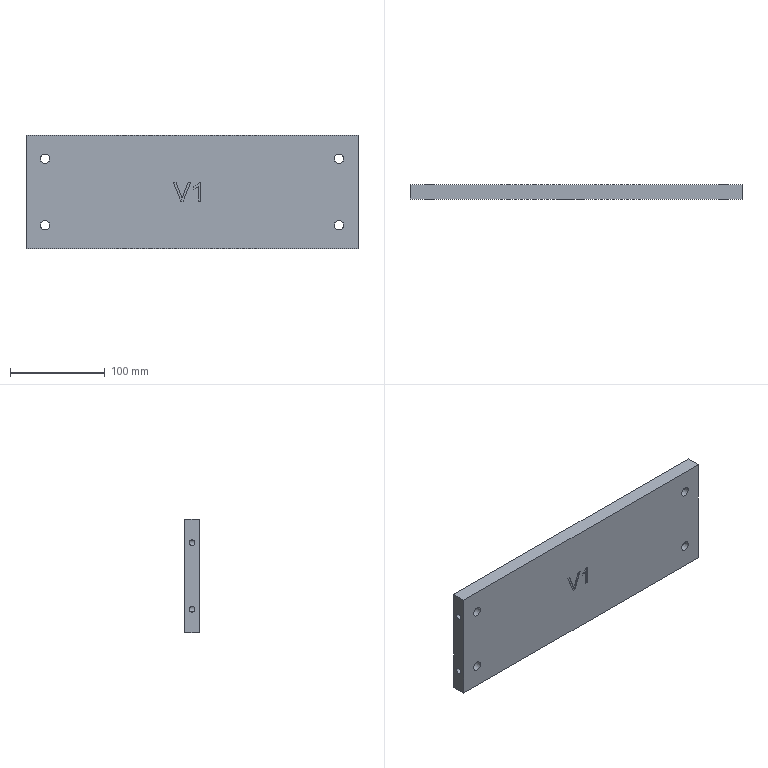Part | STEP file | Substructure | 1 solid | 34 faces | box 350 x 15 x 120 mm | volume 623484 mm3 | plane 20 | cylinder 8 | other 6 | commonest cylinder face diameters 6 x4 10 x4